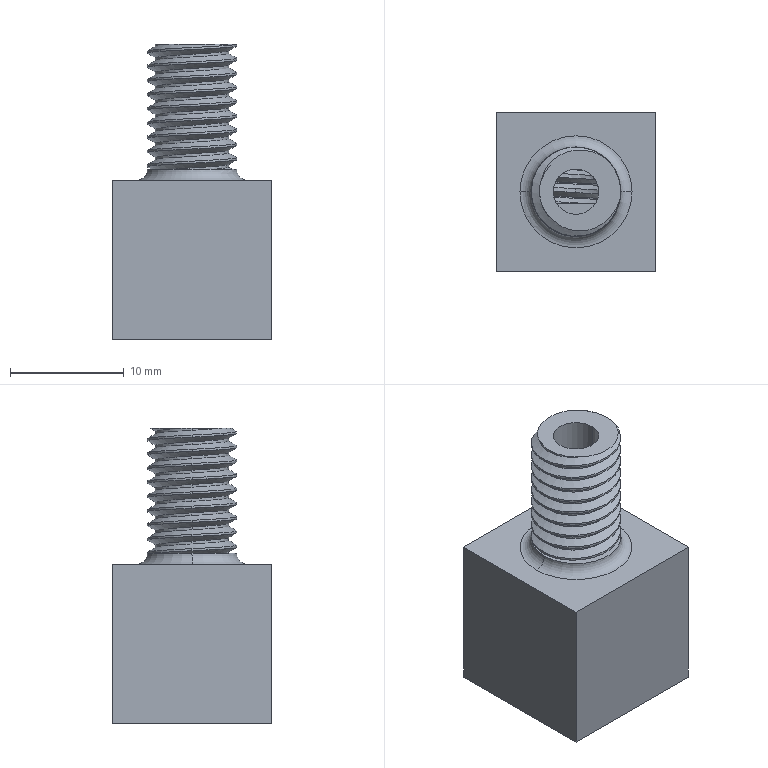Part | SolidWorks | features BaseBody 1 | 1 solid | 89 faces | volume 2700 mm3 | cylinder 68 | plane 10 | spline 9 | torus 2 | commonest cylinder face diameters 7.866 x19 6.446 x18 8.17 x14 6.779 x11 6.78 x3 4 x2